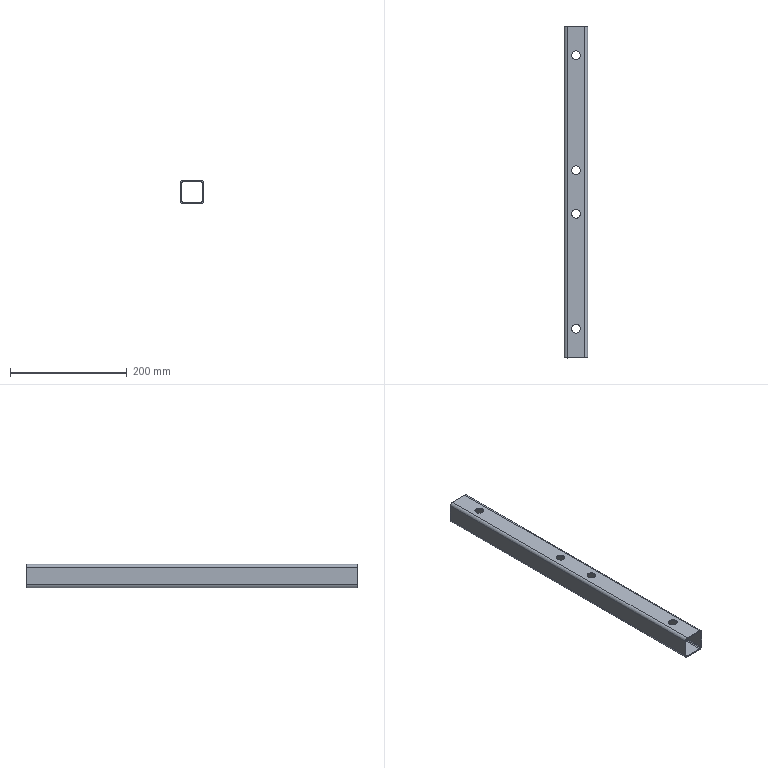Part | NX | features BREP 1 | 1 solid | 52 faces | box 40 x 568.999 x 40 mm | volume 162331 mm3 | cylinder 28 | plane 24 | commonest cylinder face diameters 15 x16 6 x8 10 x4